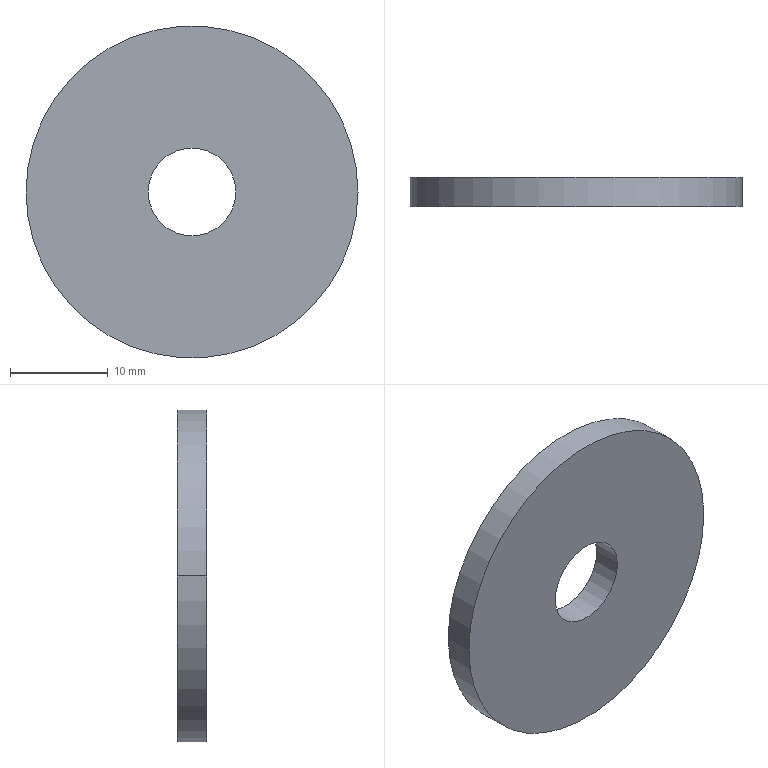Part | STEP file | LM-05-1261B | 1 solid | 6 faces | box 34 x 3 x 34 mm | volume 2533 mm3 | cylinder 4 | plane 2 | commonest cylinder face diameters 9 x2 34 x2
STEP:
#1=CARTESIAN_POINT('',(0.,0.,0.));
#2=DIRECTION('',(0.,0.,1.));
#3=DIRECTION('',(1.,0.,0.));
#4=AXIS2_PLACEMENT_3D('',#1,#2,#3);
#5=CARTESIAN_POINT('',(4.5,1.5,0.));
#6=VERTEX_POINT('',#5);
#7=CARTESIAN_POINT('',(4.5,-1.5,0.));
#8=VERTEX_POINT('',#7);
#9=CARTESIAN_POINT('',(4.5,1.5,0.));
#10=DIRECTION('',(0.,-1.,0.));
#11=VECTOR('',#10,1.);
#12=LINE('',#9,#11);
#13=CARTESIAN_POINT('',(0.,1.5,0.));
#14=DIRECTION('',(0.,-1.,0.));
#15=DIRECTION('',(1.,0.,0.));
#16=AXIS2_PLACEMENT_3D('',#13,#14,#15);
#17=CYLINDRICAL_SURFACE('',#16,4.5);
#18=CARTESIAN_POINT('',(6.283,0.));
#19=DIRECTION('',(0.,1.));
#20=VECTOR('',#19,1.);
#21=LINE('',#18,#20);
#22=(GEOMETRIC_REPRESENTATION_CONTEXT(2)PARAMETRIC_REPRESENTATION_CONTEXT()REPRESENTATION_CONTEXT('',''));
#23=DEFINITIONAL_REPRESENTATION('',(#21),#22);
#24=PCURVE('',#17,#23);
#25=CARTESIAN_POINT('',(0.,1.5,0.));
#26=DIRECTION('',(0.,-1.,0.));
#27=DIRECTION('',(1.,0.,0.));
#28=AXIS2_PLACEMENT_3D('',#25,#26,#27);
#29=CYLINDRICAL_SURFACE('',#28,4.5);
#30=CARTESIAN_POINT('',(0.,0.));
#31=DIRECTION('',(0.,1.));
#32=VECTOR('',#31,1.);
#33=LINE('',#30,#32);
#34=(GEOMETRIC_REPRESENTATION_CONTEXT(2)PARAMETRIC_REPRESENTATION_CONTEXT()REPRESENTATION_CONTEXT('',''));
#35=DEFINITIONAL_REPRESENTATION('',(#33),#34);
#36=PCURVE('',#29,#35);
#37=SURFACE_CURVE('',#12,(#24,#36),.PCURVE_S1.);
#38=EDGE_CURVE('',#6,#8,#37,.T.);
#39=ORIENTED_EDGE('',*,*,#38,.T.);
#40=CARTESIAN_POINT('',(-4.5,-1.5,0.));
#41=VERTEX_POINT('',#40);
#42=CARTESIAN_POINT('',(0.,-1.5,0.));
#43=DIRECTION('',(0.,-1.,0.));
#44=DIRECTION('',(1.,0.,0.));
#45=AXIS2_PLACEMENT_3D('',#42,#43,#44);
#46=CIRCLE('',#45,4.5);
#47=CARTESIAN_POINT('',(0.,3.));
#48=DIRECTION('',(1.,0.));
#49=VECTOR('',#48,1.);
#50=LINE('',#47,#49);
#51=(GEOMETRIC_REPRESENTATION_CONTEXT(2)PARAMETRIC_REPRESENTATION_CONTEXT()REPRESENTATION_CONTEXT('',''));
#52=DEFINITIONAL_REPRESENTATION('',(#50),#51);
#53=PCURVE('',#17,#52);
#54=CARTESIAN_POINT('',(4.5,-1.5,0.));
#55=DIRECTION('',(0.,-1.,0.));
#56=DIRECTION('',(1.,0.,0.));
#57=AXIS2_PLACEMENT_3D('',#54,#55,#56);
#58=PLANE('',#57);
#59=CARTESIAN_POINT('',(-4.5,0.));
#60=DIRECTION('',(1.,0.));
#61=AXIS2_PLACEMENT_2D('',#59,#60);
#62=CIRCLE('',#61,4.5);
#63=(GEOMETRIC_REPRESENTATION_CONTEXT(2)PARAMETRIC_REPRESENTATION_CONTEXT()REPRESENTATION_CONTEXT('',''));
#64=DEFINITIONAL_REPRESENTATION('',(#62),#63);
#65=PCURVE('',#58,#64);
#66=SURFACE_CURVE('',#46,(#53,#65),.PCURVE_S1.);
#67=EDGE_CURVE('',#41,#8,#66,.T.);
#68=ORIENTED_EDGE('',*,*,#67,.F.);
#69=CARTESIAN_POINT('',(-4.5,1.5,0.));
#70=VERTEX_POINT('',#69);
#71=CARTESIAN_POINT('',(-4.5,1.5,0.));
#72=DIRECTION('',(0.,-1.,0.));
#73=VECTOR('',#72,1.);
#74=LINE('',#71,#73);
#75=CARTESIAN_POINT('',(3.142,0.));
#76=DIRECTION('',(0.,1.));
#77=VECTOR('',#76,1.);
#78=LINE('',#75,#77);
#79=(GEOMETRIC_REPRESENTATION_CONTEXT(2)PARAMETRIC_REPRESENTATION_CONTEXT()REPRESENTATION_CONTEXT('',''));
#80=DEFINITIONAL_REPRESENTATION('',(#78),#79);
#81=PCURVE('',#17,#80);
#82=CARTESIAN_POINT('',(3.142,0.));
#83=DIRECTION('',(0.,1.));
#84=VECTOR('',#83,1.);
#85=LINE('',#82,#84);
#86=(GEOMETRIC_REPRESENTATION_CONTEXT(2)PARAMETRIC_REPRESENTATION_CONTEXT()REPRESENTATION_CONTEXT('',''));
#87=DEFINITIONAL_REPRESENTATION('',(#85),#86);
#88=PCURVE('',#29,#87);
#89=SURFACE_CURVE('',#74,(#81,#88),.PCURVE_S1.);
#90=EDGE_CURVE('',#70,#41,#89,.T.);
#91=ORIENTED_EDGE('',*,*,#90,.F.);
#92=CARTESIAN_POINT('',(0.,1.5,0.));
#93=DIRECTION('',(0.,-1.,0.));
#94=DIRECTION('',(1.,0.,0.));
#95=AXIS2_PLACEMENT_3D('',#92,#93,#94);
#96=CIRCLE('',#95,4.5);
#97=CARTESIAN_POINT('',(0.,0.));
#98=DIRECTION('',(1.,0.));
#99=VECTOR('',#98,1.);
#100=LINE('',#97,#99);
#101=(GEOMETRIC_REPRESENTATION_CONTEXT(2)PARAMETRIC_REPRESENTATION_CONTEXT()REPRESENTATION_CONTEXT('',''));
#102=DEFINITIONAL_REPRESENTATION('',(#100),#101);
#103=PCURVE('',#17,#102);
#104=CARTESIAN_POINT('',(17.,1.5,0.));
#105=DIRECTION('',(0.,1.,0.));
#106=DIRECTION('',(-1.,0.,0.));
#107=AXIS2_PLACEMENT_3D('',#104,#105,#106);
#108=PLANE('',#107);
#109=CARTESIAN_POINT('',(12.5,0.));
#110=CARTESIAN_POINT('',(12.5,7.794));
#111=CARTESIAN_POINT('',(19.25,3.897));
#112=CARTESIAN_POINT('',(26.,0.));
#113=CARTESIAN_POINT('',(19.25,-3.897));
#114=CARTESIAN_POINT('',(12.5,-7.794));
#115=CARTESIAN_POINT('',(12.5,0.));
#116=(BOUNDED_CURVE()B_SPLINE_CURVE(2,(#109,#110,#111,#112,#113,#114,#115),.UNSPECIFIED.,.T.,.F.)B_SPLINE_CURVE_WITH_KNOTS((1,2,2,2,2,1),(-2.094,0.,2.094,4.189,6.283,8.378),.UNSPECIFIED.)CURVE()GEOMETRIC_REPRESENTATION_ITEM()RATIONAL_B_SPLINE_CURVE((1.,0.5,1.,0.5,1.,0.5,1.))REPRESENTATION_ITEM(''));
#117=(GEOMETRIC_REPRESENTATION_CONTEXT(2)PARAMETRIC_REPRESENTATION_CONTEXT()REPRESENTATION_CONTEXT('',''));
#118=DEFINITIONAL_REPRESENTATION('',(#116),#117);
#119=PCURVE('',#108,#118);
#120=SURFACE_CURVE('',#96,(#103,#119),.PCURVE_S1.);
#121=EDGE_CURVE('',#70,#6,#120,.T.);
#122=ORIENTED_EDGE('',*,*,#121,.T.);
#123=EDGE_LOOP('',(#39,#68,#91,#122));
#124=FACE_BOUND('',#123,.F.);
#125=ADVANCED_FACE('',(#124),#17,.F.);
#126=CARTESIAN_POINT('',(17.,1.5,0.));
#127=VERTEX_POINT('',#126);
#128=CARTESIAN_POINT('',(-17.,1.5,0.));
#129=VERTEX_POINT('',#128);
#130=CARTESIAN_POINT('',(0.,1.5,0.));
#131=DIRECTION('',(0.,-1.,0.));
#132=DIRECTION('',(1.,0.,0.));
#133=AXIS2_PLACEMENT_3D('',#130,#131,#132);
#134=CIRCLE('',#133,17.);
#135=CARTESIAN_POINT('',(0.,1.5,0.));
#136=DIRECTION('',(0.,-1.,0.));
#137=DIRECTION('',(1.,0.,0.));
#138=AXIS2_PLACEMENT_3D('',#135,#136,#137);
#139=CYLINDRICAL_SURFACE('',#138,17.);
#140=CARTESIAN_POINT('',(0.,0.));
#141=DIRECTION('',(1.,0.));
#142=VECTOR('',#141,1.);
#143=LINE('',#140,#142);
#144=(GEOMETRIC_REPRESENTATION_CONTEXT(2)PARAMETRIC_REPRESENTATION_CONTEXT()REPRESENTATION_CONTEXT('',''));
#145=DEFINITIONAL_REPRESENTATION('',(#143),#144);
#146=PCURVE('',#139,#145);
#147=CARTESIAN_POINT('',(0.,0.));
#148=CARTESIAN_POINT('',(0.,29.445));
#149=CARTESIAN_POINT('',(25.5,14.722));
#150=CARTESIAN_POINT('',(51.,0.));
#151=CARTESIAN_POINT('',(25.5,-14.722));
#152=CARTESIAN_POINT('',(0.,-29.445));
#153=CARTESIAN_POINT('',(0.,0.));
#154=(BOUNDED_CURVE()B_SPLINE_CURVE(2,(#147,#148,#149,#150,#151,#152,#153),.UNSPECIFIED.,.T.,.F.)B_SPLINE_CURVE_WITH_KNOTS((1,2,2,2,2,1),(-2.094,0.,2.094,4.189,6.283,8.378),.UNSPECIFIED.)CURVE()GEOMETRIC_REPRESENTATION_ITEM()RATIONAL_B_SPLINE_CURVE((1.,0.5,1.,0.5,1.,0.5,1.))REPRESENTATION_ITEM(''));
#155=(GEOMETRIC_REPRESENTATION_CONTEXT(2)PARAMETRIC_REPRESENTATION_CONTEXT()REPRESENTATION_CONTEXT('',''));
#156=DEFINITIONAL_REPRESENTATION('',(#154),#155);
#157=PCURVE('',#108,#156);
#158=SURFACE_CURVE('',#134,(#146,#157),.PCURVE_S1.);
#159=EDGE_CURVE('',#127,#129,#158,.T.);
#160=ORIENTED_EDGE('',*,*,#159,.T.);
#161=CARTESIAN_POINT('',(-17.,-1.5,0.));
#162=VERTEX_POINT('',#161);
#163=CARTESIAN_POINT('',(-17.,1.5,0.));
#164=DIRECTION('',(0.,-1.,0.));
#165=VECTOR('',#164,1.);
#166=LINE('',#163,#165);
#167=CARTESIAN_POINT('',(3.142,0.));
#168=DIRECTION('',(0.,1.));
#169=VECTOR('',#168,1.);
#170=LINE('',#167,#169);
#171=(GEOMETRIC_REPRESENTATION_CONTEXT(2)PARAMETRIC_REPRESENTATION_CONTEXT()REPRESENTATION_CONTEXT('',''));
#172=DEFINITIONAL_REPRESENTATION('',(#170),#171);
#173=PCURVE('',#139,#172);
#174=CARTESIAN_POINT('',(0.,1.5,0.));
#175=DIRECTION('',(0.,-1.,0.));
#176=DIRECTION('',(1.,0.,0.));
#177=AXIS2_PLACEMENT_3D('',#174,#175,#176);
#178=CYLINDRICAL_SURFACE('',#177,17.);
#179=CARTESIAN_POINT('',(3.142,0.));
#180=DIRECTION('',(0.,1.));
#181=VECTOR('',#180,1.);
#182=LINE('',#179,#181);
#183=(GEOMETRIC_REPRESENTATION_CONTEXT(2)PARAMETRIC_REPRESENTATION_CONTEXT()REPRESENTATION_CONTEXT('',''));
#184=DEFINITIONAL_REPRESENTATION('',(#182),#183);
#185=PCURVE('',#178,#184);
#186=SURFACE_CURVE('',#166,(#173,#185),.PCURVE_S1.);
#187=EDGE_CURVE('',#129,#162,#186,.T.);
#188=ORIENTED_EDGE('',*,*,#187,.T.);
#189=CARTESIAN_POINT('',(17.,-1.5,0.));
#190=VERTEX_POINT('',#189);
#191=CARTESIAN_POINT('',(0.,-1.5,0.));
#192=DIRECTION('',(0.,-1.,0.));
#193=DIRECTION('',(1.,0.,0.));
#194=AXIS2_PLACEMENT_3D('',#191,#192,#193);
#195=CIRCLE('',#194,17.);
#196=CARTESIAN_POINT('',(0.,3.));
#197=DIRECTION('',(1.,0.));
#198=VECTOR('',#197,1.);
#199=LINE('',#196,#198);
#200=(GEOMETRIC_REPRESENTATION_CONTEXT(2)PARAMETRIC_REPRESENTATION_CONTEXT()REPRESENTATION_CONTEXT('',''));
#201=DEFINITIONAL_REPRESENTATION('',(#199),#200);
#202=PCURVE('',#139,#201);
#203=CARTESIAN_POINT('',(-4.5,0.));
#204=DIRECTION('',(1.,0.));
#205=AXIS2_PLACEMENT_2D('',#203,#204);
#206=CIRCLE('',#205,17.);
#207=(GEOMETRIC_REPRESENTATION_CONTEXT(2)PARAMETRIC_REPRESENTATION_CONTEXT()REPRESENTATION_CONTEXT('',''));
#208=DEFINITIONAL_REPRESENTATION('',(#206),#207);
#209=PCURVE('',#58,#208);
#210=SURFACE_CURVE('',#195,(#202,#209),.PCURVE_S1.);
#211=EDGE_CURVE('',#190,#162,#210,.T.);
#212=ORIENTED_EDGE('',*,*,#211,.F.);
#213=CARTESIAN_POINT('',(17.,1.5,0.));
#214=DIRECTION('',(0.,-1.,0.));
#215=VECTOR('',#214,1.);
#216=LINE('',#213,#215);
#217=CARTESIAN_POINT('',(0.,0.));
#218=DIRECTION('',(0.,1.));
#219=VECTOR('',#218,1.);
#220=LINE('',#217,#219);
#221=(GEOMETRIC_REPRESENTATION_CONTEXT(2)PARAMETRIC_REPRESENTATION_CONTEXT()REPRESENTATION_CONTEXT('',''));
#222=DEFINITIONAL_REPRESENTATION('',(#220),#221);
#223=PCURVE('',#139,#222);
#224=CARTESIAN_POINT('',(6.283,0.));
#225=DIRECTION('',(0.,1.));
#226=VECTOR('',#225,1.);
#227=LINE('',#224,#226);
#228=(GEOMETRIC_REPRESENTATION_CONTEXT(2)PARAMETRIC_REPRESENTATION_CONTEXT()REPRESENTATION_CONTEXT('',''));
#229=DEFINITIONAL_REPRESENTATION('',(#227),#228);
#230=PCURVE('',#178,#229);
#231=SURFACE_CURVE('',#216,(#223,#230),.PCURVE_S1.);
#232=EDGE_CURVE('',#127,#190,#231,.T.);
#233=ORIENTED_EDGE('',*,*,#232,.F.);
#234=EDGE_LOOP('',(#160,#188,#212,#233));
#235=FACE_BOUND('',#234,.T.);
#236=ADVANCED_FACE('',(#235),#139,.T.);
#237=ORIENTED_EDGE('',*,*,#211,.T.);
#238=CARTESIAN_POINT('',(0.,-1.5,0.));
#239=DIRECTION('',(0.,-1.,0.));
#240=DIRECTION('',(1.,0.,0.));
#241=AXIS2_PLACEMENT_3D('',#238,#239,#240);
#242=CIRCLE('',#241,17.);
#243=CARTESIAN_POINT('',(-4.5,0.));
#244=DIRECTION('',(1.,0.));
#245=AXIS2_PLACEMENT_2D('',#243,#244);
#246=CIRCLE('',#245,17.);
#247=(GEOMETRIC_REPRESENTATION_CONTEXT(2)PARAMETRIC_REPRESENTATION_CONTEXT()REPRESENTATION_CONTEXT('',''));
#248=DEFINITIONAL_REPRESENTATION('',(#246),#247);
#249=PCURVE('',#58,#248);
#250=CARTESIAN_POINT('',(0.,3.));
#251=DIRECTION('',(1.,0.));
#252=VECTOR('',#251,1.);
#253=LINE('',#250,#252);
#254=(GEOMETRIC_REPRESENTATION_CONTEXT(2)PARAMETRIC_REPRESENTATION_CONTEXT()REPRESENTATION_CONTEXT('',''));
#255=DEFINITIONAL_REPRESENTATION('',(#253),#254);
#256=PCURVE('',#178,#255);
#257=SURFACE_CURVE('',#242,(#249,#256),.PCURVE_S1.);
#258=EDGE_CURVE('',#162,#190,#257,.T.);
#259=ORIENTED_EDGE('',*,*,#258,.T.);
#260=EDGE_LOOP('',(#237,#259));
#261=FACE_BOUND('',#260,.T.);
#262=CARTESIAN_POINT('',(0.,-1.5,0.));
#263=DIRECTION('',(0.,-1.,0.));
#264=DIRECTION('',(1.,0.,0.));
#265=AXIS2_PLACEMENT_3D('',#262,#263,#264);
#266=CIRCLE('',#265,4.5);
#267=CARTESIAN_POINT('',(-4.5,0.));
#268=DIRECTION('',(1.,0.));
#269=AXIS2_PLACEMENT_2D('',#267,#268);
#270=CIRCLE('',#269,4.5);
#271=(GEOMETRIC_REPRESENTATION_CONTEXT(2)PARAMETRIC_REPRESENTATION_CONTEXT()REPRESENTATION_CONTEXT('',''));
#272=DEFINITIONAL_REPRESENTATION('',(#270),#271);
#273=PCURVE('',#58,#272);
#274=CARTESIAN_POINT('',(0.,3.));
#275=DIRECTION('',(1.,0.));
#276=VECTOR('',#275,1.);
#277=LINE('',#274,#276);
#278=(GEOMETRIC_REPRESENTATION_CONTEXT(2)PARAMETRIC_REPRESENTATION_CONTEXT()REPRESENTATION_CONTEXT('',''));
#279=DEFINITIONAL_REPRESENTATION('',(#277),#278);
#280=PCURVE('',#29,#279);
#281=SURFACE_CURVE('',#266,(#273,#280),.PCURVE_S1.);
#282=EDGE_CURVE('',#8,#41,#281,.T.);
#283=ORIENTED_EDGE('',*,*,#282,.F.);
#284=ORIENTED_EDGE('',*,*,#67,.F.);
#285=EDGE_LOOP('',(#283,#284));
#286=FACE_BOUND('',#285,.T.);
#287=ADVANCED_FACE('',(#261,#286),#58,.T.);
#288=ORIENTED_EDGE('',*,*,#187,.F.);
#289=CARTESIAN_POINT('',(0.,1.5,0.));
#290=DIRECTION('',(0.,-1.,0.));
#291=DIRECTION('',(1.,0.,0.));
#292=AXIS2_PLACEMENT_3D('',#289,#290,#291);
#293=CIRCLE('',#292,17.);
#294=CARTESIAN_POINT('',(0.,0.));
#295=DIRECTION('',(1.,0.));
#296=VECTOR('',#295,1.);
#297=LINE('',#294,#296);
#298=(GEOMETRIC_REPRESENTATION_CONTEXT(2)PARAMETRIC_REPRESENTATION_CONTEXT()REPRESENTATION_CONTEXT('',''));
#299=DEFINITIONAL_REPRESENTATION('',(#297),#298);
#300=PCURVE('',#178,#299);
#301=CARTESIAN_POINT('',(0.,0.));
#302=CARTESIAN_POINT('',(0.,29.445));
#303=CARTESIAN_POINT('',(25.5,14.722));
#304=CARTESIAN_POINT('',(51.,0.));
#305=CARTESIAN_POINT('',(25.5,-14.722));
#306=CARTESIAN_POINT('',(0.,-29.445));
#307=CARTESIAN_POINT('',(0.,0.));
#308=(BOUNDED_CURVE()B_SPLINE_CURVE(2,(#301,#302,#303,#304,#305,#306,#307),.UNSPECIFIED.,.T.,.F.)B_SPLINE_CURVE_WITH_KNOTS((1,2,2,2,2,1),(-2.094,0.,2.094,4.189,6.283,8.378),.UNSPECIFIED.)CURVE()GEOMETRIC_REPRESENTATION_ITEM()RATIONAL_B_SPLINE_CURVE((1.,0.5,1.,0.5,1.,0.5,1.))REPRESENTATION_ITEM(''));
#309=(GEOMETRIC_REPRESENTATION_CONTEXT(2)PARAMETRIC_REPRESENTATION_CONTEXT()REPRESENTATION_CONTEXT('',''));
#310=DEFINITIONAL_REPRESENTATION('',(#308),#309);
#311=PCURVE('',#108,#310);
#312=SURFACE_CURVE('',#293,(#300,#311),.PCURVE_S1.);
#313=EDGE_CURVE('',#129,#127,#312,.T.);
#314=ORIENTED_EDGE('',*,*,#313,.T.);
#315=ORIENTED_EDGE('',*,*,#232,.T.);
#316=ORIENTED_EDGE('',*,*,#258,.F.);
#317=EDGE_LOOP('',(#288,#314,#315,#316));
#318=FACE_BOUND('',#317,.T.);
#319=ADVANCED_FACE('',(#318),#178,.T.);
#320=CARTESIAN_POINT('',(0.,1.5,0.));
#321=DIRECTION('',(0.,-1.,0.));
#322=DIRECTION('',(1.,0.,0.));
#323=AXIS2_PLACEMENT_3D('',#320,#321,#322);
#324=CIRCLE('',#323,4.5);
#325=CARTESIAN_POINT('',(12.5,0.));
#326=CARTESIAN_POINT('',(12.5,7.794));
#327=CARTESIAN_POINT('',(19.25,3.897));
#328=CARTESIAN_POINT('',(26.,0.));
#329=CARTESIAN_POINT('',(19.25,-3.897));
#330=CARTESIAN_POINT('',(12.5,-7.794));
#331=CARTESIAN_POINT('',(12.5,0.));
#332=(BOUNDED_CURVE()B_SPLINE_CURVE(2,(#325,#326,#327,#328,#329,#330,#331),.UNSPECIFIED.,.T.,.F.)B_SPLINE_CURVE_WITH_KNOTS((1,2,2,2,2,1),(-2.094,0.,2.094,4.189,6.283,8.378),.UNSPECIFIED.)CURVE()GEOMETRIC_REPRESENTATION_ITEM()RATIONAL_B_SPLINE_CURVE((1.,0.5,1.,0.5,1.,0.5,1.))REPRESENTATION_ITEM(''));
#333=(GEOMETRIC_REPRESENTATION_CONTEXT(2)PARAMETRIC_REPRESENTATION_CONTEXT()REPRESENTATION_CONTEXT('',''));
#334=DEFINITIONAL_REPRESENTATION('',(#332),#333);
#335=PCURVE('',#108,#334);
#336=CARTESIAN_POINT('',(0.,0.));
#337=DIRECTION('',(1.,0.));
#338=VECTOR('',#337,1.);
#339=LINE('',#336,#338);
#340=(GEOMETRIC_REPRESENTATION_CONTEXT(2)PARAMETRIC_REPRESENTATION_CONTEXT()REPRESENTATION_CONTEXT('',''));
#341=DEFINITIONAL_REPRESENTATION('',(#339),#340);
#342=PCURVE('',#29,#341);
#343=SURFACE_CURVE('',#324,(#335,#342),.PCURVE_S1.);
#344=EDGE_CURVE('',#6,#70,#343,.T.);
#345=ORIENTED_EDGE('',*,*,#344,.T.);
#346=ORIENTED_EDGE('',*,*,#121,.T.);
#347=EDGE_LOOP('',(#345,#346));
#348=FACE_BOUND('',#347,.T.);
#349=ORIENTED_EDGE('',*,*,#159,.F.);
#350=ORIENTED_EDGE('',*,*,#313,.F.);
#351=EDGE_LOOP('',(#349,#350));
#352=FACE_BOUND('',#351,.T.);
#353=ADVANCED_FACE('',(#348,#352),#108,.T.);
#354=ORIENTED_EDGE('',*,*,#282,.F.);
#355=ORIENTED_EDGE('',*,*,#38,.F.);
#356=ORIENTED_EDGE('',*,*,#344,.T.);
#357=ORIENTED_EDGE('',*,*,#90,.T.);
#358=EDGE_LOOP('',(#354,#355,#356,#357));
#359=FACE_BOUND('',#358,.F.);
#360=ADVANCED_FACE('',(#359),#29,.F.);
#361=CLOSED_SHELL('',(#125,#236,#287,#319,#353,#360));
#362=MANIFOLD_SOLID_BREP('',#361);
#363=(LENGTH_UNIT()NAMED_UNIT(*)SI_UNIT(.MILLI.,.METRE.));
#364=UNCERTAINTY_MEASURE_WITH_UNIT(LENGTH_MEASURE(0.0000001),#363,'','');
#365=(NAMED_UNIT(*)PLANE_ANGLE_UNIT()SI_UNIT($,.RADIAN.));
#366=(NAMED_UNIT(*)SI_UNIT($,.STERADIAN.)SOLID_ANGLE_UNIT());
#367=(GEOMETRIC_REPRESENTATION_CONTEXT(3)GLOBAL_UNCERTAINTY_ASSIGNED_CONTEXT((#364))GLOBAL_UNIT_ASSIGNED_CONTEXT((#363,#365,#366))REPRESENTATION_CONTEXT('',''));
#368=ADVANCED_BREP_SHAPE_REPRESENTATION('',(#4,#362),#367);